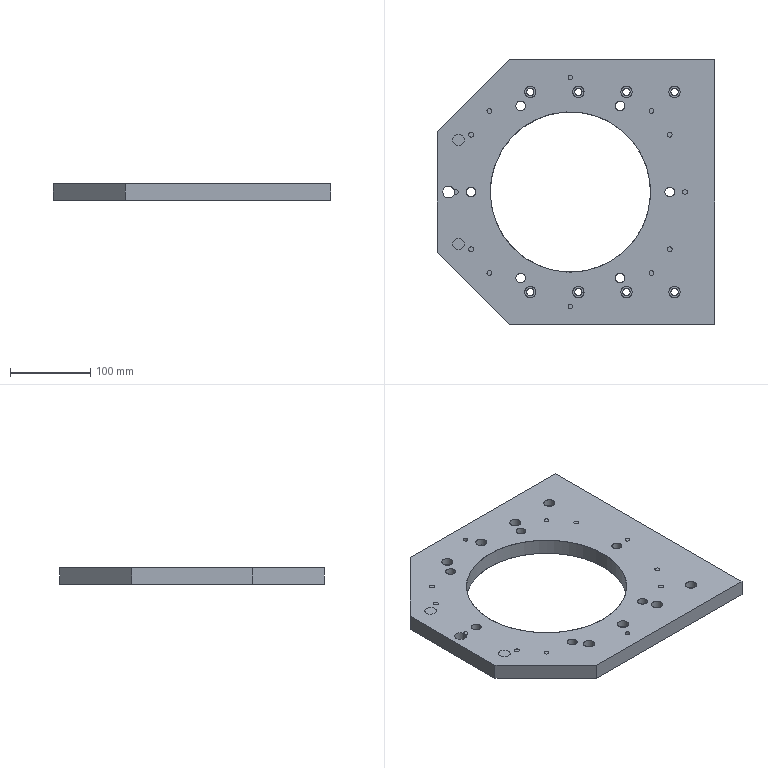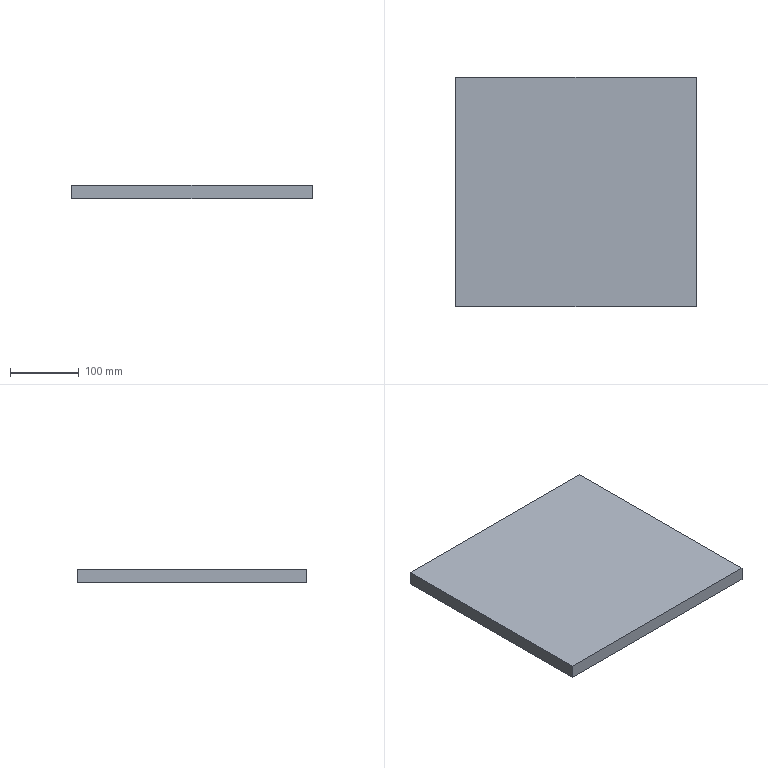CAM job | NX | 3-axis milling, drilling | part box 346 x 330 x 20 mm | stock box 350 x 334 x 20 mm
Tools:
number,name,description,diameter,corner_radius,flute_length,length,flutes
11,ZXZ,Milling Tool-5 Parameters,6.0,0.0,50.0,75.0,2
16,6.0ZT,Drilling Tool,6.0,0.0,35.0,50.0,2
19,9.0ZT,Drilling Tool,9.0,0.0,35.0,50.0,2
10,D10,Milling Tool-5 Parameters,10.0,0.0,50.0,75.0,2
6,D6,Milling Tool-5 Parameters,6.0,0.0,50.0,75.0,2
9,D10JING,Milling Tool-5 Parameters,10.0,0.0,50.0,75.0,2
7,D6A45,Milling Tool-5 Parameters,6.0,0.0,3.0,3.0,2
12,12.0ZT,Drilling Tool,12.0,0.0,35.0,50.0,2
14,14.5ZT,Drilling Tool,14.5,0.0,35.0,50.0,2
Operations:
program,operation,operation_type,tool,method,geometry_group,spindle_rpm,surface_speed,feed_per_tooth,feed_cut,feed_plunge,cut_length_mm,path_length_mm,cut_time_min,machine_time_min
CLAMP1_LR,DRILLING,Operation,ZXZ,METHOD,A,3000.0,56.0,0.0417,250.0,0.0,88.0,1462.609,0.352,0.4895
CLAMP1_LR,DRILLING_COPY,Operation,6.0ZT,METHOD,A,2000.0,37.0,0.045,180.0,0.0,88.816,1047.788,0.4934,0.5893
CLAMP1_LR,DRILLING_COPY_COPY,Operation,9.0ZT,METHOD,A,1000.0,28.0,0.09,180.0,0.0,213.631,1198.73,1.187,1.285
CLAMP1_LR,DRILLING_COPY_COPY_COPY,Operation,12.0ZT,METHOD,A,1000.0,28.0,0.09,180.0,0.0,165.631,1106.443,0.9202,1.014
CLAMP1_LR,DRILLING_COPY_COPY_COPY_COPY,Operation,14.5ZT,METHOD,A,800.0,36.0,0.1125,180.0,0.0,28.356,196.713,0.1575,0.1744
CLAMP1_LR,HOLE_MILLING,CylinderMilling,D10,METHOD,A,3200.0,100.0,0.3438,2200.0,100.0,4492.572,6290.572,2.042,2.222
CLAMP1_LR,ZLEVEL_PROFILE,ZLevelMilling,D10,METHOD,A,2200.0,69.0,0.5,2200.0,100.0,48721.931,49446.347,22.146,22.219
CLAMP1_LR,ZLEVEL_PROFILE_COPY_1,ZLevelMilling,D10,METHOD,A,2200.0,69.0,0.5,2200.0,100.0,54376.01,54532.86,24.716,24.732
CLAMP1_LR,ZLEVEL_PROFILE_COPY,ZLevelMilling,D10JING,METHOD,A,5000.0,157.0,0.12,1200.0,100.0,514.596,1238.5,0.4288,0.5012
CLAMP1_LR,ZLEVEL_PROFILE_COPY_COPY_1,ZLevelMilling,D6,METHOD,A,5000.0,157.0,0.12,1200.0,100.0,1232.024,1405.838,1.027,1.044
CLAMP1_LR,ZLEVEL_PROFILE_COPY_COPY,ZLevelMilling,D6A45,METHOD,A,7500.0,141.0,0.08,1200.0,100.0,1944.03,9429.778,1.62,2.369
CLAMP2_FB,ZLEVEL_PROFILE_COPY_1_1,ZLevelMilling,D10,METHOD,A,2200.0,69.0,0.5,2200.0,100.0,75551.231,76050.98,34.342,34.391
CLAMP2_FB,ZLEVEL_PROFILE_COPY_COPY_1_1,ZLevelMilling,D10JING,METHOD,A,5000.0,157.0,0.12,1200.0,100.0,809.008,1315.944,0.6742,0.7249
CLAMP2_FB,ZLEVEL_PROFILE_COPY_COPY_COPY,ZLevelMilling,D6A45,METHOD,A,7500.0,141.0,0.08,1200.0,100.0,792.936,1213.291,0.6608,0.7028